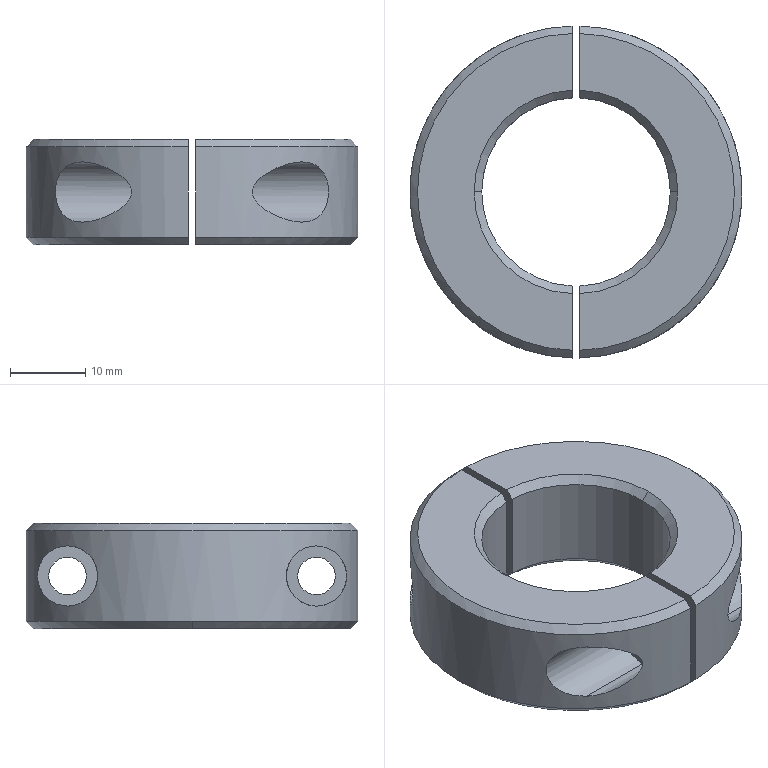Part | SolidWorks | features ICE 3, Chamfer 1, Extrusion 1, MirrorSolid 1 | 2 solids | 44 faces | box 44 x 43.989 x 14 mm | volume 11608 mm3 | cylinder 20 | cone 12 | plane 12 | commonest cylinder face diameters 5 x8 8 x8 25 x2 44 x2